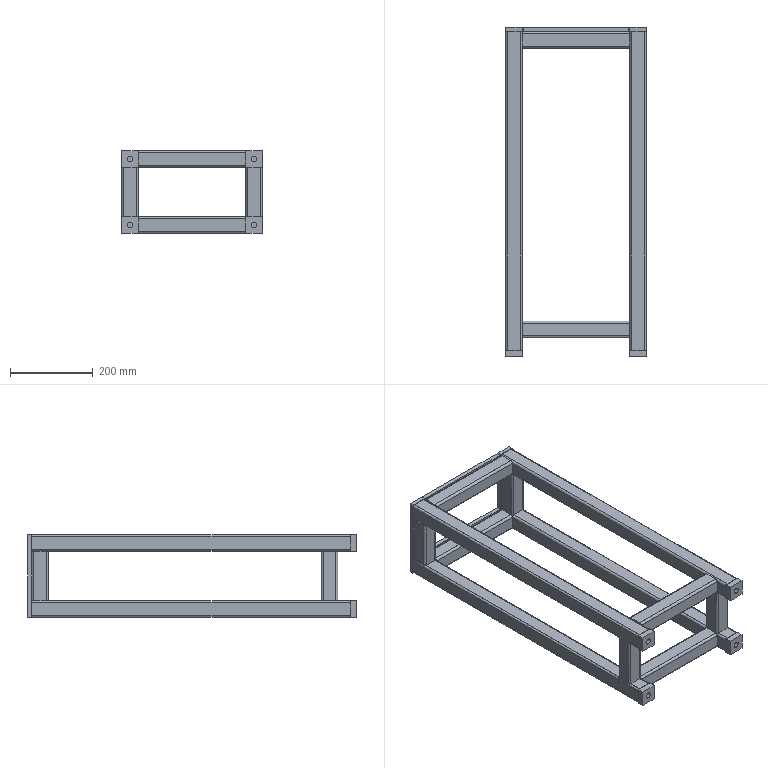Part | SolidWorks | features BaseBody 20, MoveFace 1 | 20 solids | 272 faces | box 340 x 795 x 200 mm | volume 2102526 mm3 | plane 168 | cylinder 104 | commonest cylinder face diameters 5 x48 10 x48 14 x8